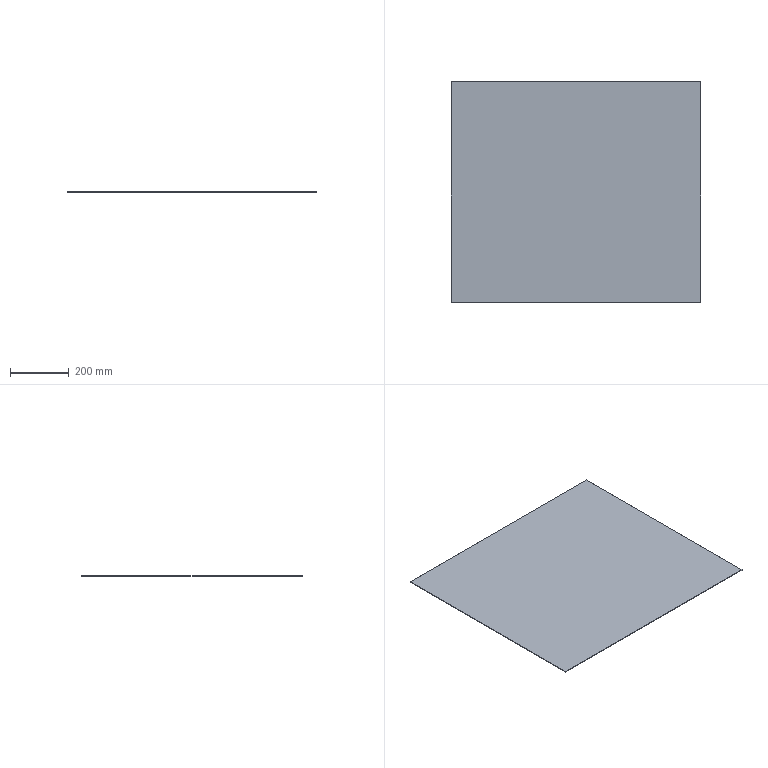Part | STEP file | Upper frame acrylic side plate | 1 solid | 6 faces | box 848.001 x 747.917 x 2 mm | volume 1268468 mm3 | plane 6
STEP:
#1=CARTESIAN_POINT('',(0.,0.,0.));
#2=VERTEX_POINT('',#1);
#3=CARTESIAN_POINT('',(0.,-747.917,0.));
#4=VERTEX_POINT('',#3);
#5=CARTESIAN_POINT('',(0.,0.,0.));
#6=DIRECTION('',(0.,-1.,0.));
#7=VECTOR('',#6,1000.);
#8=LINE('',#5,#7);
#9=EDGE_CURVE('',#2,#4,#8,.T.);
#10=ORIENTED_EDGE('',*,*,#9,.T.);
#11=CARTESIAN_POINT('',(0.,-747.917,2.));
#12=VERTEX_POINT('',#11);
#13=CARTESIAN_POINT('',(0.,-747.917,2.));
#14=DIRECTION('',(0.,0.,-1.));
#15=VECTOR('',#14,1000.);
#16=LINE('',#13,#15);
#17=EDGE_CURVE('',#12,#4,#16,.T.);
#18=ORIENTED_EDGE('',*,*,#17,.F.);
#19=CARTESIAN_POINT('',(0.,0.,2.));
#20=VERTEX_POINT('',#19);
#21=CARTESIAN_POINT('',(0.,0.,2.));
#22=DIRECTION('',(0.,-1.,0.));
#23=VECTOR('',#22,1000.);
#24=LINE('',#21,#23);
#25=EDGE_CURVE('',#20,#12,#24,.T.);
#26=ORIENTED_EDGE('',*,*,#25,.F.);
#27=CARTESIAN_POINT('',(0.,0.,2.));
#28=DIRECTION('',(0.,0.,-1.));
#29=VECTOR('',#28,1000.);
#30=LINE('',#27,#29);
#31=EDGE_CURVE('',#20,#2,#30,.T.);
#32=ORIENTED_EDGE('',*,*,#31,.T.);
#33=EDGE_LOOP('',(#10,#18,#26,#32));
#34=FACE_OUTER_BOUND('',#33,.T.);
#35=CARTESIAN_POINT('',(0.,0.,2.));
#36=DIRECTION('',(1.,0.,0.));
#37=DIRECTION('',(0.,1.,0.));
#38=AXIS2_PLACEMENT_3D('',#35,#36,#37);
#39=PLANE('',#38);
#40=ADVANCED_FACE('',(#34),#39,.F.);
#41=CARTESIAN_POINT('',(848.001,-747.917,0.));
#42=VERTEX_POINT('',#41);
#43=CARTESIAN_POINT('',(0.,-747.917,0.));
#44=DIRECTION('',(1.,0.,0.));
#45=VECTOR('',#44,1000.);
#46=LINE('',#43,#45);
#47=EDGE_CURVE('',#4,#42,#46,.T.);
#48=ORIENTED_EDGE('',*,*,#47,.T.);
#49=CARTESIAN_POINT('',(848.001,-747.917,2.));
#50=VERTEX_POINT('',#49);
#51=CARTESIAN_POINT('',(848.001,-747.917,2.));
#52=DIRECTION('',(0.,0.,-1.));
#53=VECTOR('',#52,1000.);
#54=LINE('',#51,#53);
#55=EDGE_CURVE('',#50,#42,#54,.T.);
#56=ORIENTED_EDGE('',*,*,#55,.F.);
#57=CARTESIAN_POINT('',(0.,-747.917,2.));
#58=DIRECTION('',(1.,0.,0.));
#59=VECTOR('',#58,1000.);
#60=LINE('',#57,#59);
#61=EDGE_CURVE('',#12,#50,#60,.T.);
#62=ORIENTED_EDGE('',*,*,#61,.F.);
#63=ORIENTED_EDGE('',*,*,#17,.T.);
#64=EDGE_LOOP('',(#48,#56,#62,#63));
#65=FACE_OUTER_BOUND('',#64,.T.);
#66=CARTESIAN_POINT('',(0.,-747.917,2.));
#67=DIRECTION('',(0.,1.,0.));
#68=DIRECTION('',(0.,0.,1.));
#69=AXIS2_PLACEMENT_3D('',#66,#67,#68);
#70=PLANE('',#69);
#71=ADVANCED_FACE('',(#65),#70,.F.);
#72=CARTESIAN_POINT('',(848.001,0.,0.));
#73=VERTEX_POINT('',#72);
#74=CARTESIAN_POINT('',(848.001,0.,0.));
#75=DIRECTION('',(0.,1.,0.));
#76=VECTOR('',#75,1000.);
#77=LINE('',#74,#76);
#78=EDGE_CURVE('',#42,#73,#77,.T.);
#79=ORIENTED_EDGE('',*,*,#78,.T.);
#80=CARTESIAN_POINT('',(848.001,0.,2.));
#81=VERTEX_POINT('',#80);
#82=CARTESIAN_POINT('',(848.001,0.,2.));
#83=DIRECTION('',(0.,0.,-1.));
#84=VECTOR('',#83,1000.);
#85=LINE('',#82,#84);
#86=EDGE_CURVE('',#81,#73,#85,.T.);
#87=ORIENTED_EDGE('',*,*,#86,.F.);
#88=CARTESIAN_POINT('',(848.001,0.,2.));
#89=DIRECTION('',(0.,1.,0.));
#90=VECTOR('',#89,1000.);
#91=LINE('',#88,#90);
#92=EDGE_CURVE('',#50,#81,#91,.T.);
#93=ORIENTED_EDGE('',*,*,#92,.F.);
#94=ORIENTED_EDGE('',*,*,#55,.T.);
#95=EDGE_LOOP('',(#79,#87,#93,#94));
#96=FACE_OUTER_BOUND('',#95,.T.);
#97=CARTESIAN_POINT('',(848.001,0.,2.));
#98=DIRECTION('',(-1.,0.,0.));
#99=DIRECTION('',(0.,-1.,0.));
#100=AXIS2_PLACEMENT_3D('',#97,#98,#99);
#101=PLANE('',#100);
#102=ADVANCED_FACE('',(#96),#101,.F.);
#103=CARTESIAN_POINT('',(0.,0.,0.));
#104=DIRECTION('',(-1.,0.,0.));
#105=VECTOR('',#104,1000.);
#106=LINE('',#103,#105);
#107=EDGE_CURVE('',#73,#2,#106,.T.);
#108=ORIENTED_EDGE('',*,*,#107,.T.);
#109=ORIENTED_EDGE('',*,*,#31,.F.);
#110=CARTESIAN_POINT('',(0.,0.,2.));
#111=DIRECTION('',(-1.,0.,0.));
#112=VECTOR('',#111,1000.);
#113=LINE('',#110,#112);
#114=EDGE_CURVE('',#81,#20,#113,.T.);
#115=ORIENTED_EDGE('',*,*,#114,.F.);
#116=ORIENTED_EDGE('',*,*,#86,.T.);
#117=EDGE_LOOP('',(#108,#109,#115,#116));
#118=FACE_OUTER_BOUND('',#117,.T.);
#119=CARTESIAN_POINT('',(0.,0.,2.));
#120=DIRECTION('',(0.,-1.,0.));
#121=DIRECTION('',(0.,0.,-1.));
#122=AXIS2_PLACEMENT_3D('',#119,#120,#121);
#123=PLANE('',#122);
#124=ADVANCED_FACE('',(#118),#123,.F.);
#125=ORIENTED_EDGE('',*,*,#25,.T.);
#126=ORIENTED_EDGE('',*,*,#61,.T.);
#127=ORIENTED_EDGE('',*,*,#92,.T.);
#128=ORIENTED_EDGE('',*,*,#114,.T.);
#129=EDGE_LOOP('',(#125,#126,#127,#128));
#130=FACE_OUTER_BOUND('',#129,.T.);
#131=CARTESIAN_POINT('',(0.,0.,2.));
#132=DIRECTION('',(0.,0.,1.));
#133=DIRECTION('',(1.,0.,0.));
#134=AXIS2_PLACEMENT_3D('',#131,#132,#133);
#135=PLANE('',#134);
#136=ADVANCED_FACE('',(#130),#135,.T.);
#137=ORIENTED_EDGE('',*,*,#9,.F.);
#138=ORIENTED_EDGE('',*,*,#107,.F.);
#139=ORIENTED_EDGE('',*,*,#78,.F.);
#140=ORIENTED_EDGE('',*,*,#47,.F.);
#141=EDGE_LOOP('',(#137,#138,#139,#140));
#142=FACE_OUTER_BOUND('',#141,.T.);
#143=CARTESIAN_POINT('',(0.,0.,0.));
#144=DIRECTION('',(0.,0.,1.));
#145=DIRECTION('',(1.,0.,0.));
#146=AXIS2_PLACEMENT_3D('',#143,#144,#145);
#147=PLANE('',#146);
#148=ADVANCED_FACE('',(#142),#147,.F.);
#149=CLOSED_SHELL('',(#40,#71,#102,#124,#136,#148));
#150=MANIFOLD_SOLID_BREP('',#149);
#151=CARTESIAN_POINT('',(0.,0.,0.));
#152=DIRECTION('',(0.,0.,1.));
#153=DIRECTION('',(1.,0.,0.));
#154=AXIS2_PLACEMENT_3D('',#151,#152,#153);
#155=(LENGTH_UNIT()NAMED_UNIT(*)SI_UNIT(.MILLI.,.METRE.));
#156=UNCERTAINTY_MEASURE_WITH_UNIT(LENGTH_MEASURE(0.00001),#155,'','');
#157=(NAMED_UNIT(*)PLANE_ANGLE_UNIT()SI_UNIT($,.RADIAN.));
#158=(NAMED_UNIT(*)SI_UNIT($,.STERADIAN.)SOLID_ANGLE_UNIT());
#159=(GEOMETRIC_REPRESENTATION_CONTEXT(3)GLOBAL_UNCERTAINTY_ASSIGNED_CONTEXT((#156))GLOBAL_UNIT_ASSIGNED_CONTEXT((#155,#157,#158))REPRESENTATION_CONTEXT('',''));
#160=ADVANCED_BREP_SHAPE_REPRESENTATION('',(#150,#154),#159);